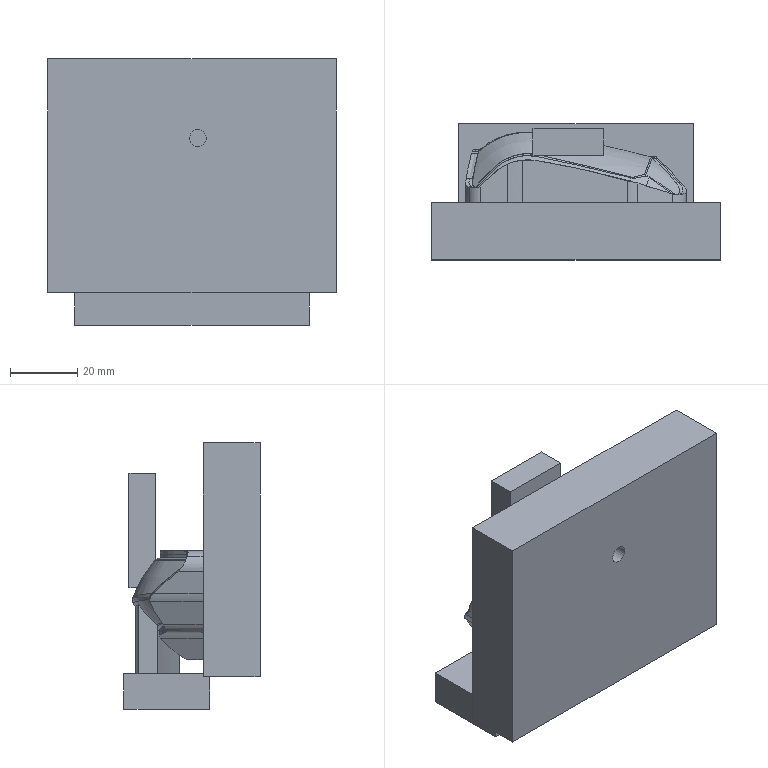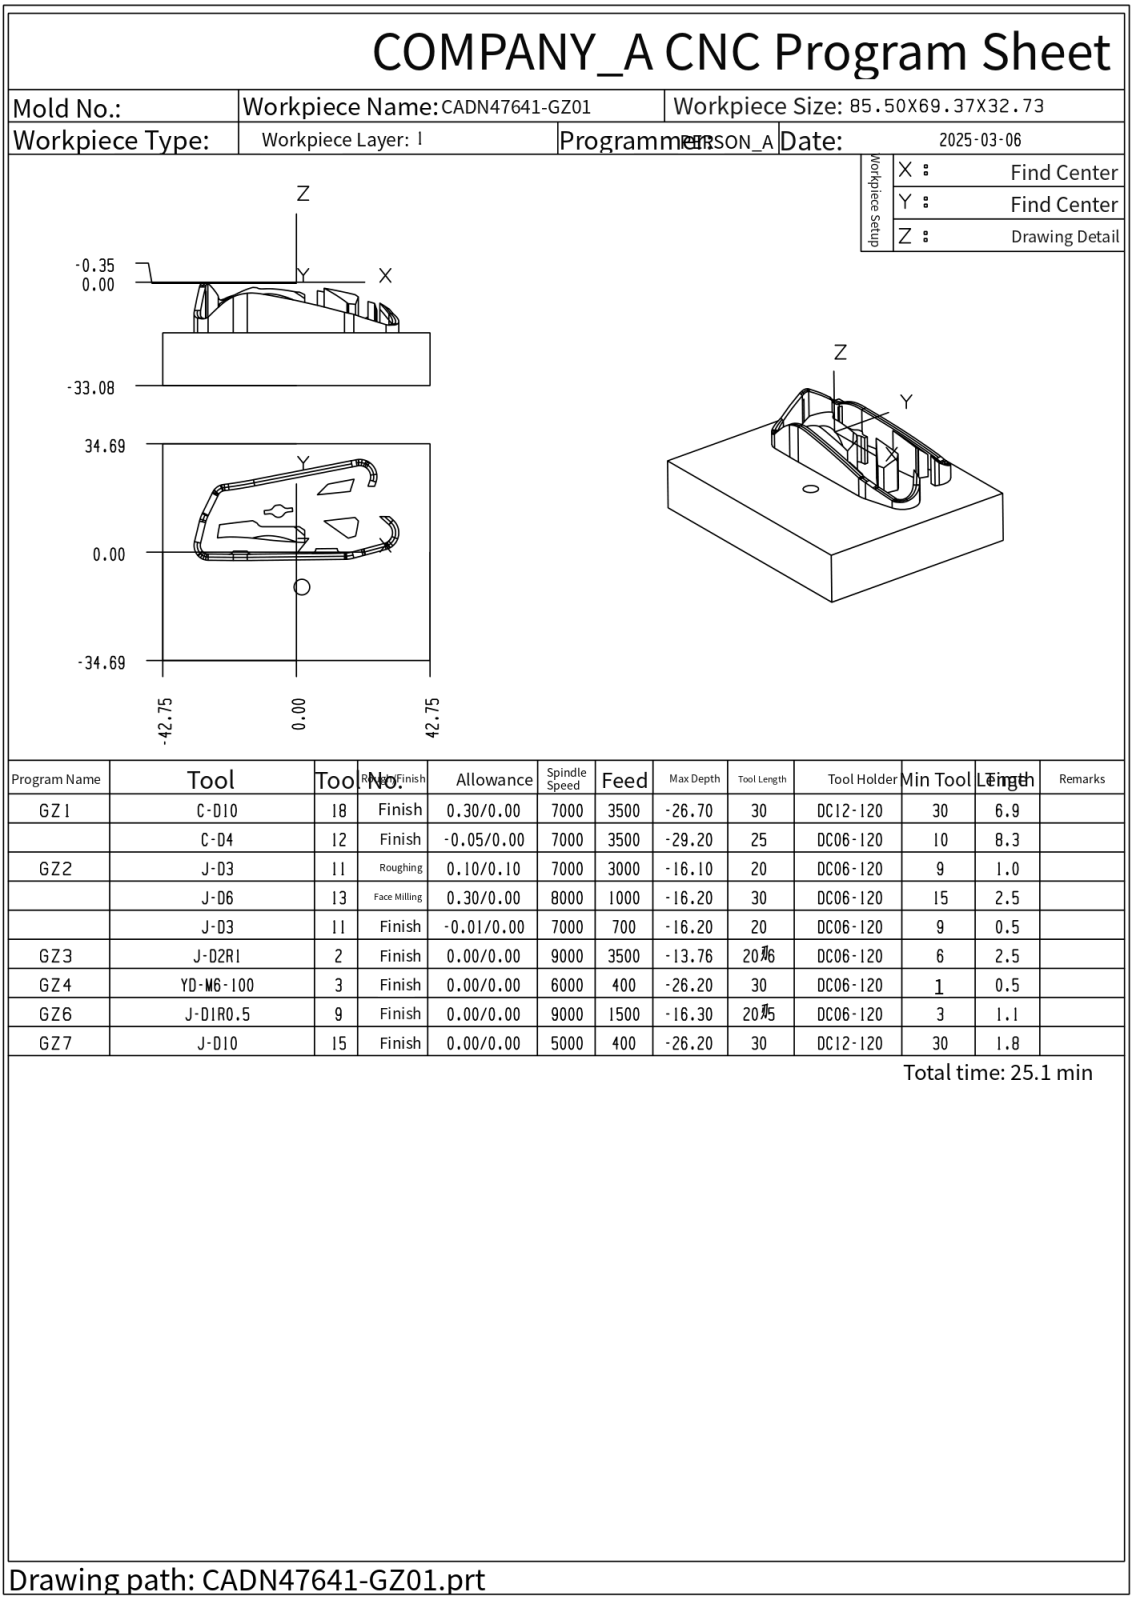NC program | NX | posted by the shop | part box 85.5 x 40.385 x 79 mm
Lines 36040 to 36898 of 71032:
36039 TOOL CALL 10 Z S7000
36040 CALL LBL101
36041 M3 M8
36042 M51
36043 CYCL DEF 32.0 TOLERANCE
36044 CYCL DEF 32.1 T0.012
36045 CYCL DEF 32.2 HSC-MODE:0
36046 L M126
36047 PLANE SPATIAL SPA-90. SPB+0.0 SPC+180. TURN FMAX SEQ-
36048 L X24.8955 Y1.6366 FMAX
36049 L Z102.5 FMAX
36050 L Z8.2072 FMAX
36051 L Z7.2072 F1500.
36052 CC X25.3717 Y2.5159
36053 C X26.2511 Y2.0397 DR+
36054 CC X27.7805 Y1.2115
36055 C X26.3392 Y2.1851 DR- F3000.
36056 L X26.3096 Y2.2798
36057 L X26.2417 Y2.5151
36058 L X26.1261 Y2.3992 Z7.1574
36059 L X26.0636 Y2.3031 Z7.1076
36060 L X26.1734 Y2.0672
36061 CC X27.7778 Y1.1917
36062 C X26.084 Y1.8786 DR+
36063 L X26.0215 Y1.8443 Z7.0579
36064 L X25.9513 Y1.813 Z7.0081
36065 CC X27.3487 Y1.2565
36066 C X26.0344 Y1.9878 DR-
36067 L X25.8966 Y2.2389
36068 L X25.8145 Y2.2304 Z6.9583
36069 L X25.7429 Y2.2281 Z6.9085
36070 L X25.797 Y2.1394
36071 L X25.9108 Y1.9375
36072 CC X27.42 Y1.2131
36073 C X25.8323 Y1.744 DR+
36074 L X25.7242 Y1.7093 Z6.8089
36075 CC X27.5017 Y1.1601
36076 C X25.7986 Y1.9087 DR-
36077 L X25.6495 Y2.143
36078 L X25.5344 Y2.1299 Z6.7094
36079 L X25.692 Y1.8917
36080 CC X27.1996 Y1.2027
36081 C X25.6196 Y1.7037 DR+
36082 L X25.5195 Y1.7021 Z6.6098
36083 CC X27.3098 Y1.2067
36084 C X25.5856 Y1.8979 DR-
36085 CC X33.768 Y7.9039
36086 C X25.4478 Y2.0903 DR-
36087 L X25.339 Y2.1081 Z6.5102
36088 L X25.489 Y1.8865
36089 CC X26.9832 Y1.2052
36090 C X25.4181 Y1.7025 DR+
36091 L X25.3164 Y1.6861 Z6.4106
36092 CC X27.0085 Y1.1978
36093 C X25.3883 Y1.888 DR-
36094 CC X39.6492 Y12.0493
36095 C X25.2447 Y2.0926 DR-
36096 L X25.1426 Y2.0958 Z6.3111
36097 CC X41.4267 Y13.3714
36098 C X25.2873 Y1.8897 DR+
36099 CC X26.8851 Y1.196
36100 C X25.2153 Y1.6919 DR+
36101 L X25.114 Y1.6927 Z6.2115
36102 CC X26.8865 Y1.1603
36103 C X25.1863 Y1.8914 DR-
36104 L X25.0346 Y2.1137
36105 L X24.938 Y2.1018 Z6.1119
36106 CC X43.0434 Y14.724
36107 C X25.0853 Y1.8931 DR+
36108 CC X26.6853 Y1.1961
36109 C X25.0125 Y1.6936 DR+
36110 L X24.9108 Y1.6893 Z6.0123
36111 CC X26.7839 Y1.1358
36112 C X24.9842 Y1.8947 DR-
36113 CC X43.0304 Y14.8684
36114 C X24.8355 Y2.1041 DR-
36115 L X24.7258 Y2.1236 Z5.9128
36116 L X24.8832 Y1.8963
36117 CC X26.4842 Y1.1965
36118 C X24.8094 Y1.6947 DR+
36119 L X24.7079 Y1.695 Z5.8132
36120 CC X26.385 Y1.1965
36121 C X24.7819 Y1.8974 DR-
36122 CC X46.4901 Y17.538
36123 C X24.6298 Y2.1107 DR-
36124 L X24.5174 Y2.1339 Z5.7136
36125 L X24.6805 Y1.8982
36126 CC X26.2829 Y1.1968
36127 C X24.6055 Y1.6929 DR+
36128 L X24.5528 Y1.698 Z5.6638
36129 L X24.5034 Y1.7028 Z5.614
36130 CC X26.0829 Y1.2061
36131 C X24.5791 Y1.8991 DR-
36132 L X24.4146 Y2.1348
36133 L X24.3127 Y2.1338 Z5.5145
36134 L X24.4766 Y1.9005
36135 CC X26.3028 Y1.1302
36136 C X24.4006 Y1.6872 DR+
36137 L X24.2982 Y1.6896 Z5.4149
36138 CC X26.2077 Y1.1283
36139 C X24.374 Y1.9021 DR-
36140 L X24.2106 Y2.1327
36141 L X24.1056 Y2.1354 Z5.3153
36142 L X24.2712 Y1.9035
36143 CC X25.8632 Y1.1994
36144 C X24.1945 Y1.6952 DR+
36145 L X24.0904 Y1.6843 Z5.2157
36146 CC X25.8194 Y1.2023
36147 C X24.1675 Y1.9045 DR-
36148 CC X52.3731 Y22.7661
36149 C X24.0075 Y2.1226 DR-
36150 L X23.8997 Y2.1319 Z5.1162
36151 L X24.0639 Y1.9054
36152 CC X25.8639 Y1.1348
36153 C X23.9869 Y1.6921 DR+
36154 L X23.9317 Y1.6946 Z5.0664
36155 L X23.8831 Y1.6967 Z5.0166
36156 CC X25.558 Y1.1996
36157 C X23.9603 Y1.9064 DR-
36158 L X23.7961 Y2.1315
36159 L X23.6907 Y2.1351 Z4.917
36160 L X23.8567 Y1.9074
36161 CC X25.4562 Y1.1996
36162 C X23.7791 Y1.6964 DR+
36163 L X23.675 Z4.8174
36164 CC X25.3517 Y1.1999
36165 C X23.7531 Y1.9084 DR-
36166 CC X-14.5661 Y-25.5947
36167 C X23.5828 Y2.1441 DR+
36168 L X23.4754 Y2.1519 Z4.7179
36169 CC X6.3711 Y-10.3123
36170 C X23.6495 Y1.9095 DR-
36171 CC X25.2481 Y1.2001
36172 C X23.571 Y1.6963 DR+
36173 L X23.4661 Y1.6939 Z4.6183
36174 CC X25.1407 Y1.2006
36175 C X23.5459 Y1.9105 DR-
36176 L X23.3701 Y2.1518
36177 L X23.2597 Y2.1585 Z4.5187
36178 L X23.4422 Y1.9115
36179 CC X25.0281 Y1.2006
36180 C X23.3603 Y1.6892 DR+
36181 L X23.2545 Y1.6872 Z4.4192
36182 CC X24.9323 Y1.2016
36183 C X23.3369 Y1.9127 DR-
36184 CC X-1.8278 Y-16.8967
36185 C X23.1545 Y2.1544 DR+
36186 L X23.0463 Y2.1564 Z4.3196
36187 CC X1.77 Y-14.2955
36188 C X23.2316 Y1.9139 DR-
36189 CC X25.0476 Y1.1316
36190 C X23.1486 Y1.6829 DR+
36191 L X23.0416 Y1.6845 Z4.22
36192 CC X24.7127 Y1.2029
36193 C X23.1258 Y1.9145 DR-
36194 CC X12.7774 Y-5.7107
36195 C X22.9256 Y2.179 DR+
36196 L X22.818 Y2.1742 Z4.1204
36197 CC X10.7984 Y-7.3342
36198 C X23.0192 Y1.9142 DR-
36199 CC X24.4819 Y1.2153
36200 C X22.9339 Y1.6967 DR+
36201 L X22.8259 Y1.6771 Z4.0209
36202 CC X24.4887 Y1.2027
36203 C X22.9125 Y1.9139 DR-
36204 CC X14.3973 Y-4.4789
36205 C X22.702 Y2.1851 DR+
36206 L X22.6044 Y2.1613 Z3.9213
36207 CC X10.6334 Y-7.7466
36208 C X22.8045 Y1.9144 DR-
36209 CC X24.238 Y1.2167
36210 C X22.7182 Y1.6983 DR+
36211 L X22.6063 Y1.6673 Z3.8217
36212 CC X24.2788 Y1.205
36213 C X22.6958 Y1.9155 DR-
36214 CC X15.3362 Y-3.7929
36215 C X22.4727 Y2.1921 DR+
36216 L X22.3547 Y2.1969 Z3.7221
36217 CC X15.6882 Y-3.55
36218 C X22.5868 Y1.9161 DR-
36219 CC X24.1608 Y1.2043
36220 C X22.4946 Y1.6606 DR+
36221 L X22.383 Y1.6581 Z3.6226
36222 CC X24.0143 Y1.211
36223 C X22.4759 Y1.914 DR-
36224 CC X16.2269 Y-3.0782
36225 C X22.2405 Y2.1952 DR+
36226 L X22.1209 Y2.196 Z3.523
36227 CC X16.4218 Y-2.9462
36228 C X22.365 Y1.9119 DR-
36229 CC X24.4735 Y1.0454
36230 C X22.2684 Y1.6235 DR+
36231 L X22.2135 Y1.6281 Z3.4732
36232 L X22.1524 Y1.6331 Z3.4234
36233 CC X23.7678 Y1.2112
36234 C X22.2516 Y1.9104 DR-
36235 CC X16.4952 Y-2.9147
36236 C X21.9929 Y2.2032 DR+
36237 L X21.8711 Y2.2002 Z3.3238
36238 CC X16.515 Y-2.9538
36239 C X22.1363 Y1.9095 DR-
36240 CC X23.6864 Y1.2123
36241 C X22.0357 Y1.617 DR+
36242 L X21.9832 Y1.621 Z3.2741
36243 L X21.9192 Y1.6259 Z3.2243
36244 CC X23.5139 Y1.2118
36245 C X22.0208 Y1.9083 DR-
36246 CC X16.5828 Y-2.9487
36247 C X21.7491 Y2.1964 DR+
36248 L X21.6213 Y2.1893 Z3.1247
36249 CC X15.2422 Y-4.4418
36250 C X21.9036 Y1.9056 DR-
36251 CC X23.3745 Y1.2115
36252 C X21.7979 Y1.6111 DR+
36253 L X21.676 Y1.5633 Z3.0251
36254 CC X23.3595 Y1.2036
36255 C X21.7864 Y1.9028 DR-
36256 CC X16.3602 Y-3.34
36257 C X21.4761 Y2.206 DR+
36258 L X21.364 Y2.1765 Z2.9255
36259 CC X15.043 Y-4.9679
36260 C X21.6638 Y1.8996 DR-
36261 CC X23.199 Y1.2006
36262 C X21.5553 Y1.5796 DR+
36263 L X21.4271 Y1.5614 Z2.826
36264 CC X23.0389 Y1.2097
36265 C X21.539 Y1.8966 DR-
36266 CC X16.0115 Y-3.928
36267 C X21.2034 Y2.1976 DR+
36268 L X21.1256 Y2.2076 Z2.7762
36269 L X21.044 Y2.213 Z2.7264
36270 CC X17.09 Y-2.7001
36271 C X21.4127 Y1.892 DR-
36272 CC X22.8976 Y1.2075
36273 C X21.2973 Y1.5432 DR+
36274 L X21.2325 Y1.5413 Z2.6766
36275 L X21.1674 Y1.5394 Z2.6268
36276 CC X22.7246 Y1.2057
36277 C X21.2845 Y1.8859 DR-
36278 CC X16.3127 Y-3.7358
36279 C X20.9148 Y2.1923 DR+
36280 L X20.8438 Y2.192 Z2.577
36281 L X20.7692 Y2.187 Z2.5272
36282 CC X16.8294 Y-3.1385
36283 C X21.1542 Y1.8794 DR-
36284 CC X22.5922 Y1.205
36285 C X21.0365 Y1.5251 DR+
36286 L X20.9669 Y1.5 Z2.4775
36287 L X20.8978 Y1.4747 Z2.4277
36288 CC X22.5262 Y1.2043
36289 C X21.0171 Y1.8732 DR-
36290 CC X16.7702 Y-3.2507
36291 C X20.6072 Y2.187 DR+
36292 L X20.5297 Y2.1862 Z2.3779
36293 L X20.449 Y2.1808 Z2.3281
36294 CC X16.723 Y-3.3841
36295 C X20.8796 Y1.867 DR-
36296 CC X22.2455 Y1.2033
36297 C X20.7555 Y1.4967 DR+
36298 L X20.6775 Y1.4875 Z2.2783
36299 L X20.6106 Y1.4761 Z2.2285
36300 CC X22.0897 Y1.1998
36301 C X20.7376 Y1.8599 DR-
36302 CC X16.3511 Y-4.0036
36303 C X20.2744 Y2.1795 DR+
36304 L X20.1978 Y2.1727 Z2.1787
36305 L X20.1182 Y2.1612 Z2.129
36306 CC X15.7622 Y-5.0156
36307 C X20.5933 Y1.8503 DR-
36308 CC X21.9683 Y1.1963
36309 C X20.4662 Y1.4456 DR+
36310 L X20.3884 Y1.4336 Z2.0792
36311 L X20.3209 Y1.4199 Z2.0294
36312 CC X21.8815 Y1.1977
36313 C X20.4425 Y1.8411 DR-
36314 CC X16.212 Y-4.3432
36315 C X19.9557 Y2.1473 DR+
36316 L X19.8655 Y2.1439 Z1.9796
36317 L X19.7731 Y2.1364 Z1.9298
36318 CC X15.6636 Y-5.3909
36319 C X20.2883 Y1.8313 DR-
36320 CC X21.6455 Y1.1962
36321 C X20.1601 Y1.3939 DR+
36322 L X20.0692 Y1.3996 Z1.88
36323 L X19.9965 Y1.4041 Z1.8302
36324 CC X21.4189 Y1.1858
36325 C X20.1279 Y1.8214 DR-
36326 CC X16.4847 Y-3.9749
36327 C X19.5825 Y2.1303 DR+
36328 L X19.5031 Y2.1175 Z1.7804
36329 L X19.4219 Y2.1009 Z1.7307
36330 CC X16.11 Y-4.7151
36331 C X19.9624 Y1.8107 DR-
36332 CC X21.2876 Y1.1796
36333 C X19.8345 Y1.3871 DR+
36334 L X19.7466 Y1.3778 Z1.6809
36335 L X19.6662 Y1.3675 Z1.6311
36336 CC X21.1125 Y1.1767
36337 C X19.7934 Y1.7999 DR-
36338 CC X15.6865 Y-5.6573
36339 C X19.2476 Y2.0754 DR+
36340 L X19.1513 Y2.0682 Z1.5813
36341 L X19.0546 Y2.0601 Z1.5315
36342 CC X15.3276 Y-6.4919
36343 C X19.6171 Y1.7923 DR-
36344 CC X20.8571 Y1.187
36345 C X19.4896 Y1.3712 DR+
36346 L X19.3836 Y1.36 Z1.4815
36347 L X19.2953 Y1.3506 Z1.4315
36348 CC X20.7028 Y1.1833
36349 C X19.4179 Y1.7818 DR-
36350 CC X15.4281 Y-6.3559
36351 C X18.834 Y2.0429 DR+
36352 L X18.7398 Y2.0287 Z1.3815
36353 L X18.6442 Y2.0108 Z1.3315
36354 CC X14.683 Y-8.3264
36355 C X19.2262 Y1.7686 DR-
36356 CC X20.5094 Y1.1784
36357 C X19.1067 Y1.3437 DR+
36358 L X19.0013 Y1.3284 Z1.2815
36359 L X18.8998 Y1.3137 Z1.2315
36360 CC X20.2832 Y1.197
36361 C X19.014 Y1.7597 DR-
36362 CC X14.1995 Y-9.874
36363 C X18.4142 Y1.9902 DR+
36364 L X18.3087 Y1.9791 Z1.1815
36365 L X18.1998 Y1.9579 Z1.1315
36366 CC X13.469 Y-12.3197
36367 C X18.7953 Y1.7466 DR-
36368 CC X20.0777 Y1.1937
36369 C X18.6858 Y1.308 DR+
36370 L X18.5782 Y1.2926 Z1.0815
36371 L X18.4657 Y1.2765 Z1.0315
36372 CC X19.8461 Y1.1892
36373 C X18.5732 Y1.7304 DR-
36374 CC X12.9417 Y-14.567
36375 C X17.9606 Y1.9293 DR+
36376 L X17.868 Y1.9315 Z.9982
36377 L X17.7727 Y1.9243 Z.9648
36378 L X17.6775 Y1.917 Z.9315
36379 CC X14.6835 Y-9.0695
36380 C X18.3307 Y1.7178 DR-
36381 CC X19.6265 Y1.202
36382 C X18.2328 Y1.2543 DR+
36383 L X18.1102 Y1.2385 Z.8815
36384 L X17.9775 Y1.2214 Z.8315
36385 CC X19.3484 Y1.2017
36386 C X18.0722 Y1.7029 DR-
36387 CC X12.8002 Y-16.2613
36388 C X17.4204 Y1.8815 DR+
36389 L X17.3247 Y1.8752 Z.7982
36390 L X17.228 Y1.8648 Z.7648
36391 L X17.1312 Y1.8534 Z.7315
36392 CC X13.994 Y-12.2062
36393 C X17.8124 Y1.6838 DR-
36394 CC X19.0577 Y1.1906
36395 C X17.7183 Y1.1954 DR+
36396 L X17.5837 Y1.1765 Z.6815
36397 L X17.4321 Y1.1552 Z.6315
36398 CC X18.8845 Y1.1988
36399 C X17.5088 Y1.6666 DR-
36400 L X17.2415 Y1.7336
36401 L X16.8502 Y1.8072
36402 L X16.7445 Y1.8025 Z.5982
36403 L X16.6373 Y1.7902 Z.5648
36404 L X16.5299 Y1.7761 Z.5315
36405 CC X11.3526 Y-27.6509
36406 C X17.2129 Y1.6477 DR-
36407 CC X18.4403 Y1.1985
36408 C X17.1349 Y1.1335 DR+
36409 L X16.9452 Y1.1091 Z.4821
36410 L X16.7844 Y1.0886 Z.4328
36411 CC X18.0507 Y1.1999
36412 C X16.8524 Y1.6238 DR-
36413 L X16.678 Y1.6584
36414 L X16.162 Y1.7294
36415 L X16.0563 Y1.7271 Z.4081
36416 L X15.9497 Y1.7179 Z.3834
36417 L X15.8429 Y1.7069 Z.3587
36418 L X15.736 Y1.6949 Z.334
36419 CC X11.6675 Y-32.4141
36420 C X16.4749 Y1.5986 DR-
36421 CC X17.6471 Y1.1903
36422 C X16.4113 Y1.0745 DR+
36423 L X16.1834 Y1.0708 Z.2847
36424 L X15.9657 Y1.0672 Z.2353
36425 CC X17.0647 Y1.1989
36426 C X16.0222 Y1.5708 DR-
36427 CC X10.9722 Y-47.6625
36428 C X15.2909 Y1.6404 DR+
36429 L X15.1694 Y1.6278 Z.2106
36430 L X15.0477 Y1.6117 Z.1859
36431 L X14.9259 Y1.5957 Z.1612
36432 L X14.8037 Y1.5714 Z.1365
36433 L X15.2694 Y1.5538
36434 L X15.5005 Y1.5348
36435 CC X16.6876 Y1.2266
36436 C X15.4836 Y.9926 DR+
36437 CC X14.502 Y.8019
36438 C X14.6927 Y-.1798 DR-
36439 L Z1.1365
36440 L Z11.6923 FMAX
36441 L X28.5933 Y5.6856 F10000.
36442 L Z8.2072 FMAX
36443 L Z7.2072 F1500.
36444 CC X29.2913 Y4.9696
36445 C X28.5753 Y4.2715 DR+
36446 CC X27.2359 Y2.9659
36447 C X28.7776 Y4.0249 DR- F3000.
36448 CC X29.0636 Y6.0509
36449 C X29.3278 Y4.022 DR+
36450 L X29.3899 Y4.0662 Z7.1574
36451 L X29.4516 Y4.113 Z7.1076
36452 L X29.3559 Y4.1072
36453 CC X29.2696 Y5.1375
36454 C X29.0018 Y4.1388 DR-
36455 CC X27.9022 Y3.6327
36456 C X28.8866 Y4.3371 DR+
36457 L X28.9658 Y4.3912 Z7.0579
36458 L X29.0391 Y4.4413 Z7.0081
36459 CC X28.0269 Y3.7013
36460 C X29.1639 Y4.23 DR-
36461 CC X29.432 Y5.0372
36462 C X29.498 Y4.1892 DR+
36463 CC X29.6697 Y1.9821
36464 C X29.6155 Y4.1952 DR-
36465 L X29.6185 Y4.2308 Z6.9583
36466 L X29.6216 Y4.2667 Z6.9085
36467 CC X29.6187 Y1.6606
36468 C X29.4498 Y4.2613 DR+
36469 L X29.2844 Y4.3076
36470 L X29.2462 Y4.3858
36471 L X29.1363 Y4.5334
36472 L X29.2173 Y4.5518 Z6.8587
36473 L X29.2817 Y4.5586 Z6.8089
36474 CC X28.1765 Y3.8131
36475 C X29.382 Y4.3825 DR-
36476 L X29.4443 Y4.36
36477 CC X29.8709 Y6.4386
36478 C X29.7986 Y4.3179 DR+
36479 L X29.77 Y4.3977 Z6.7094
36480 L X29.6376 Y4.4008
36481 CC X29.6242 Y4.7303
36482 C X29.4587 Y4.4451 DR-
36483 CC X28.4493 Y3.9997
36484 C X29.3681 Y4.6104 DR+
36485 L X29.398 Y4.6405 Z6.6596
36486 L X29.4291 Y4.6717 Z6.6098
36487 CC X28.6175 Y4.0992
36488 C X29.5238 Y4.5054 DR-
36489 CC X29.6446 Y4.6706
36490 C X29.6376 Y4.4661 DR+
36491 L X29.7785 Y4.461
36492 CC X20.6695 Y-82.9604
36493 C X29.9096 Y4.4473 DR-
36494 L X29.8666 Y4.5179 Z6.5102
36495 CC X29.3458 Y-1.6371
36496 C X29.6376 Y4.533 DR+
36497 L X29.5913 Y4.5594
36498 L X29.5865 Y4.5593
36499 CC X28.4884 Y3.9865
36500 C X29.4906 Y4.7142 DR+
36501 L X29.5218 Y4.7731 Z6.4106
36502 CC X27.6309 Y3.2691
36503 C X29.634 Y4.62 DR-
36504 CC X29.7112 Y4.7067
36505 C X29.7141 Y4.5906 DR+
36506 L X29.7785 Y4.588
36507 L X29.9377 Y4.5757
36508 L X30.0164 Y4.5986 Z6.3608
36509 L X30.094 Y4.6375 Z6.3111
36510 CC X30.5563 Y2.2835
36511 C X30.0607 Y4.6307 DR+
36512 L X29.7785 Y4.6515
36513 L X29.71 Y4.6541
36514 L X29.5441 Y4.8375
36515 L X29.5278 Y4.9264 Z6.2115
36516 L X29.7137 Y4.7211
36517 L X30.0146 Y4.6991
36518 CC X30.5758 Y2.8323
36519 C X30.1067 Y4.7244 DR-
36520 L X30.1436 Y4.813 Z6.1119
36521 CC X30.7465 Y2.1282
36522 C X29.9757 Y4.7697 DR+
36523 L X29.7073 Y4.7892
36524 L X29.6376 Y4.8633
36525 L X29.5077 Y5.0104
36526 L X29.4743 Y5.1047 Z6.0123
36527 L X29.6376 Y4.9195
36528 L X29.6948 Y4.8575
36529 L X29.9311 Y4.8384
36530 CC X30.801 Y2.2297
36531 C X30.165 Y4.9051 DR-
36532 L X30.1448 Y4.9438 Z5.9625
36533 L X30.1263 Y4.9796 Z5.9128
36534 CC X30.9334 Y2.1156
36535 C X29.9066 Y4.9084 DR+
36536 L X29.6817 Y4.9259
36537 L X29.4597 Y5.178
36538 L X29.4282 Y5.2663 Z5.8132
36539 L X29.6651 Y4.9982
36540 L X29.8865 Y4.9804
36541 CC X31.1166 Y1.8536
36542 C X30.1271 Y5.0647 DR-
36543 L X30.13 Y5.1507 Z5.7136
36544 L X29.9194 Y5.0785
36545 L X29.8633 Y5.0562
36546 L X29.6469 Y5.0722
36547 L X29.5077 Y5.2282
36548 L X29.3981 Y5.3536
36549 L X29.3789 Y5.4325 Z5.614
36550 L X29.629 Y5.1461
36551 L X29.8439 Y5.1314
36552 L X30.1544 Y5.2406
36553 L X30.1466 Y5.3279 Z5.5145
36554 L X29.8177 Y5.2075
36555 L X29.7785 Y5.2121
36556 L X29.6107 Y5.2209
36557 L X29.3518 Y5.5179
36558 L X29.3259 Y5.6026 Z5.4149
36559 L X29.593 Y5.2958
36560 L X29.7911 Y5.2835
36561 L X30.1356 Y5.4134
36562 L X30.1071 Y5.456 Z5.3651
36563 L X30.0837 Y5.491 Z5.3153
36564 L X29.7645 Y5.3594
36565 L X29.5753 Y5.3707
36566 L X29.3002 Y5.6873
36567 L X29.2837 Y5.764 Z5.2157
36568 L X29.5577 Y5.4456
36569 L X29.7378 Y5.4353
36570 L X30.0802 Y5.5745
36571 L X30.0723 Y5.6196 Z5.166
36572 L X30.066 Y5.6557 Z5.1162
36573 L X29.7113 Y5.5111
36574 L X29.5399 Y5.5206
36575 CC X-14.3195 Y-31.6691
36576 C X29.2648 Y5.8427 DR+
36577 L X29.2358 Y5.9288 Z5.0166
36578 L X29.5219 Y5.5961
36579 L X29.6849 Y5.5874
36580 L X30.049 Y5.7356
36581 L X30.0202 Y5.7739 Z4.9668
36582 L X29.9951 Y5.8073 Z4.917
36583 L X29.6611 Y5.6634
36584 L X29.5038 Y5.6715
36585 L X29.4012 Y5.7898
36586 L X29.2147 Y6.0088
36587 L X29.1901 Y6.0926 Z4.8174
36588 L X29.4858 Y5.7474
36589 L X29.6404 Y5.74
36590 L X29.9856 Y5.8879
36591 L X29.9277 Y5.9588 Z4.7179
36592 CC X30.8405 Y3.5668
36593 C X29.6206 Y5.8178 DR+
36594 L X29.4671 Y5.8247
36595 L X29.1744 Y6.1678
36596 L X29.1548 Y6.2471 Z4.6183
36597 L X29.4484 Y5.902
36598 L X29.601 Y5.8955
36599 L X29.9452 Y6.0418
36600 L X29.9481 Y6.1231 Z4.5187
36601 L X29.5814 Y5.9732
36602 L X29.4297 Y5.9794
36603 L X29.1399 Y6.3228
36604 L X29.122 Y6.4009 Z4.4192
36605 L X29.4111 Y6.0567
36606 L X29.5619 Y6.0509
36607 L X29.9279 Y6.1997
36608 L X29.9036 Y6.2354 Z4.3694
36609 L X29.8789 Y6.2717 Z4.3196
36610 CC X30.9073 Y3.3952
36611 C X29.5433 Y6.1286 DR+
36612 L X29.3928 Y6.1342
36613 L X29.1055 Y6.478
36614 L X29.0863 Y6.5571 Z4.22
36615 L X29.3559 Y6.2337
36616 L X29.3745 Y6.2119
36617 L X29.525 Y6.2062
36618 L X29.9022 Y6.3554
36619 L X29.8905 Y6.3984 Z4.1702
36620 L X29.8814 Y6.4319 Z4.1204
36621 L X29.5067 Y6.2838
36622 L X29.3559 Y6.2903
36623 L X29.0693 Y6.6345
36624 L X29.0541 Y6.7106 Z4.0209
36625 L X29.3384 Y6.3679
36626 L X29.4883 Y6.3617
36627 L X29.8421 Y6.5054
36628 L X29.834 Y6.5448 Z3.9711
36629 L X29.8259 Y6.584 Z3.9213
36630 L X29.4706 Y6.4414
36631 L X29.3192 Y6.4474
36632 L X29.1637 Y6.6321
36633 L X29.0309 Y6.7939
36634 L X29.0214 Y6.8666 Z3.8217
36635 L X29.3 Y6.5269
36636 L X29.4529 Y6.5211
36637 L X29.8099 Y6.6627
36638 L X29.7607 Y6.7361 Z3.7221
36639 CC X30.5843 Y4.294
36640 C X29.4352 Y6.6008 DR+
36641 L X29.2809 Y6.6063
36642 L X28.9968 Y6.9516
36643 L X28.9772 Y7.0325 Z3.6226
36644 L X29.2617 Y6.6865
36645 L X29.4168 Y6.6809
36646 L X29.7771 Y6.8184
36647 L X29.7028 Y6.8886 Z3.523
36648 CC X30.3978 Y4.7964
36649 C X29.398 Y6.7612 DR+
36650 L X29.2424 Y6.7669
36651 L X28.9627 Y7.1093
36652 L X28.9408 Y7.1917 Z3.4234
36653 L X29.0742 Y7.0272
36654 L X29.2232 Y6.8473
36655 L X29.3809 Y6.8414
36656 L X29.723 Y6.9685
36657 L X29.7069 Y7.0049 Z3.3736
36658 L X29.6903 Y7.0423 Z3.3238
36659 CC X31.1196 Y2.6917
36660 C X29.3648 Y6.9215 DR+
36661 L X29.204 Y6.9278
36662 L X29.0742 Y7.0849
36663 L X28.9252 Y7.2689
36664 L X28.9092 Y7.3485 Z3.2243
36665 L X29.1848 Y7.0088
36666 L X29.3516 Y7.0012
36667 CC X30.6311 Y4.2129
36668 C X29.6599 Y7.123 DR-
36669 L X29.731 Y7.2187 Z3.1247
36670 L X29.3319 Y7.0818
36671 L X29.1656 Y7.0897
36672 L X28.8935 Y7.4279
36673 L X28.8753 Y7.5094 Z3.0251
36674 L X29.1464 Y7.1706
36675 L X29.3139 Y7.1627
36676 L X29.3999 Y7.1937
36677 L X29.7242 Y7.3036
36678 L X29.6474 Y7.3757 Z2.9255
36679 CC X31.0982 Y2.9594
36680 C X29.2983 Y7.2452 DR+
36681 L X29.1265 Y7.253
36682 L X28.8556 Y7.5926
36683 L X28.8361 Y7.6755 Z2.826
36684 L X29.1064 Y7.336
36685 L X29.2813 Y7.328
36686 CC X30.8376 Y3.7389
36687 C X29.6214 Y7.457 DR-
36688 L X29.6122 Y7.4969 Z2.7762
36689 L X29.6025 Y7.5394 Z2.7264
36690 L X29.2643 Y7.4107
36691 L X29.0863 Y7.419
36692 L X28.8167 Y7.7584
36693 L X28.7964 Y7.842 Z2.6268
36694 L X29.0663 Y7.5019
36695 L X29.2469 Y7.4935
36696 L X29.5834 Y7.6218
36697 L X29.5745 Y7.6607 Z2.577
36698 L X29.5645 Y7.7043 Z2.5272
36699 L X29.2289 Y7.5764
36700 L X29.0465 Y7.5851
36701 L X28.7772 Y7.925
36702 L X28.753 Y8.0131 Z2.4277
36703 L X28.9564 Y7.7553
36704 L X29.0266 Y7.6682
36705 L X29.2108 Y7.6593
36706 CC X28.281 Y10.7578
36707 C X29.5698 Y7.7906 DR+
36708 L X29.5505 Y7.8322 Z2.3779
36709 L X29.5326 Y7.8705 Z2.3281
36710 L X29.1927 Y7.7422
36711 L X29.0068 Y7.7513
36712 L X28.7352 Y8.0959
36713 L X28.7105 Y8.1845 Z2.2285
36714 L X28.7924 Y8.0788
36715 L X28.9865 Y7.8357
36716 L X29.1761 Y7.8261
36717 L X29.5163 Y7.9536
36718 L X29.4971 Y7.9907 Z2.1787
36719 L X29.4751 Y8.0334 Z2.129
36720 CC X29.9381 Y6.9529
36721 C X29.3559 Y7.9741 DR+
36722 L X29.1599 Y7.9102
36723 L X28.9662 Y7.9201
36724 L X28.7021 Y8.2595
36725 L X28.6817 Y8.3448 Z2.0294
36726 L X28.9206 Y8.0361
36727 L X28.9458 Y8.0045
36728 L X29.1436 Y7.9942
36729 L X29.3559 Y8.0632
36730 L X29.482 Y8.1202
36731 L X29.4745 Y8.1632 Z1.9796
36732 L X29.4673 Y8.2048 Z1.9298
36733 CC X29.9115 Y7.1775
36734 C X29.4399 Y8.1925 DR+
36735 L X29.3559 Y8.1535
36736 L X29.1272 Y8.0789
36737 L X28.9251 Y8.0898
36738 L X28.7924 Y8.2575
36739 L X28.6563 Y8.4344
36740 L X28.643 Y8.514 Z1.8302
36741 L X28.9042 Y8.1755
36742 L X29.0742 Y8.1681
36743 L X29.1108 Y8.1641
36744 L X29.215 Y8.1976
36745 L X29.4796 Y8.294
36746 L X29.4685 Y8.3443 Z1.7804
36747 L X29.461 Y8.378 Z1.7307
36748 L X29.0943 Y8.2493
36749 L X29.0742 Y8.2515
36750 L X28.8833 Y8.2612
36751 CC X88.7079 Y55.2401
36752 C X28.6127 Y8.6079 DR-
36753 L X28.5943 Y8.6935 Z1.6311
36754 L X28.667 Y8.5977
36755 L X28.8627 Y8.347
36756 L X29.0771 Y8.3347
36757 L X29.484 Y8.4754
36758 L X29.4125 Y8.5407 Z1.5315
36759 L X29.0579 Y8.4163
36760 L X28.8436 Y8.4284
36761 L X28.7924 Y8.4939
36762 L X28.5857 Y8.7651
36763 L X28.566 Y8.8558 Z1.4315
36764 L X28.8223 Y8.5189
36765 L X29.036 Y8.507
36766 CC X32.7314 Y-1.7133
36767 C X29.4066 Y8.6335 DR-
36768 L X29.3437 Y8.7125 Z1.3315
36769 CC X30.5692 Y4.8176
36770 C X29.0152 Y8.5935 DR+
36771 L X28.802 Y8.6052
36772 L X28.5896 Y8.8785
36773 L X28.5309 Y8.9561
36774 L X28.5237 Y9.0325 Z1.2315
36775 L X28.7804 Y8.6935
36776 L X28.9992 Y8.6814
36777 L X29.3172 Y8.7975
36778 L X29.3063 Y8.8384 Z1.1815
36779 L X29.2944 Y8.8833 Z1.1315
36780 L X28.9835 Y8.7693
36781 L X28.7924 Y8.7826
36782 L X28.7585 Y8.7822
36783 L X28.6837 Y8.8785
36784 L X28.4963 Y9.1263
36785 L X28.4805 Y9.2103 Z1.0315
36786 CC X-840.2096 Y-646.5419
36787 C X28.7366 Y8.871 DR-
36788 L X28.9678 Y8.8573
36789 L X29.2766 Y8.9707
36790 L X29.2671 Y9.0132 Z.9815
36791 L X29.257 Y9.0579 Z.9315
36792 L X28.9484 Y8.9459
36793 L X28.715 Y8.9597
36794 L X28.5622 Y9.1593
36795 L X28.4552 Y9.3026
36796 L X28.4406 Y9.3855 Z.8315
36797 L X28.6935 Y9.0485
36798 L X28.928 Y9.0346
36799 CC X27.9015 Y12.5835
36800 C X29.2611 Y9.1483 DR+
36801 L X29.1931 Y9.2294 Z.7315
36802 CC X29.6449 Y8.1485
36803 C X29.0742 Y9.1716 DR+
36804 L X28.9077 Y9.1233
36805 L X28.672 Y9.1373
36806 L X28.4218 Y9.4721
36807 L X28.4019 Y9.5602 Z.6315
36808 L X28.6506 Y9.2266
36809 L X28.8898 Y9.2126
36810 CC X27.2363 Y14.7677
36811 C X29.2271 Y9.3244 DR+
36812 L X29.2209 Y9.3769 Z.5815
36813 L X29.2171 Y9.41 Z.5315
36814 CC X27.0543 Y15.4461
36815 C X28.8744 Y9.2979 DR-
36816 L X28.6301 Y9.3116
36817 L X28.3797 Y9.6471
36818 L X28.3486 Y9.7481 Z.4328
36819 L X28.3687 Y9.7209
36820 L X28.6078 Y9.4045
36821 L X28.8575 Y9.3911
36822 L X29.1809 Y9.4994
36823 L X29.1786 Y9.5896 Z.334
36824 L X28.9333 Y9.5064
36825 L X28.8401 Y9.4803
36826 L X28.5858 Y9.4941
36827 L X28.4144 Y9.7209
36828 L X28.331 Y9.8336
36829 L X28.3177 Y9.9155 Z.2353
36830 L X28.5633 Y9.5843
36831 L X28.8213 Y9.5701
36832 L X29.1517 Y9.6761
36833 L X29.1484 Y9.732 Z.1859
36834 L X29.1462 Y9.768 Z.1365
36835 CC X62.3534 Y-96.4182
36836 C X28.8025 Y9.6598 DR+
36837 L X28.5407 Y9.6746
36838 L X28.2864 Y10.0146
36839 L X28.267 Y10.1033 Z.0378
36840 L X28.3418 Y10.0017
36841 L X28.5187 Y9.7649
36842 L X28.7837 Y9.7497
36843 L X29.1492 Y9.8617
36844 L X29.0907 Y9.9442 Z-.0609
36845 L X28.7625 Y9.8401
36846 L X28.497 Y9.8552
36847 L X28.2499 Y10.1899
36848 L X28.2284 Y10.2804 Z-.1597
36849 L X28.4753 Y9.9456
36850 L X28.7413 Y9.9304
36851 CC X30.4722 Y5.1107
36852 C X29.0509 Y10.0306 DR-
36853 L X29.0262 Y10.0744 Z-.2091
36854 L X29.0023 Y10.117 Z-.2584
36855 L X28.7197 Y10.0208
36856 L X28.4533 Y10.0364
36857 L X28.2066 Y10.3714
36858 L X28.1811 Y10.4659 Z-.3572
36859 L X28.316 Y10.2825
36860 L X28.4308 Y10.1282
36861 L X28.702 Y10.1124
36862 L X28.9802 Y10.2072
36863 L X28.9935 Y10.3018 Z-.4559
36864 CC X28.203 Y12.2757
36865 C X28.6849 Y10.2048 DR-
36866 L X28.4083 Y10.2199
36867 L X28.1631 Y10.5536
36868 L X28.1383 Y10.6473 Z-.5546
36869 L X28.229 Y10.5238
36870 L X28.3858 Y10.312
36871 L X28.6723 Y10.2983
36872 L X28.941 Y10.388
36873 L X28.9887 Y10.489 Z-.6534
36874 CC X28.5198 Y11.607
36875 C X28.3631 Y10.4048 DR-
36876 L X28.2457 Y10.5633
36877 L X28.118 Y10.7372
36878 L X28.0978 Y10.8275 Z-.7521
36879 L X28.3405 Y10.4977
36880 CC X28.4949 Y11.7146
36881 C X28.7924 Y10.5245 DR+
36882 L X28.9136 Y10.5728
36883 L X28.9016 Y10.6207 Z-.8015
36884 L X28.8906 Y10.6648 Z-.8509
36885 L X28.7924 Y10.622
36886 CC X28.4681 Y11.9171
36887 C X28.3177 Y10.5905 DR-
36888 L X28.229 Y10.7093
36889 L X28.0726 Y10.9224
36890 L X28.0519 Y11.0132 Z-.9496
36891 L X28.2948 Y10.6833
36892 L X28.5735 Y10.6719
36893 L X28.6516 Y10.6858
36894 L X28.8805 Y10.7585
36895 L X28.916 Y10.867 Z-1.0484
36896 L X28.6516 Y10.7846
36897 L X28.5651 Y10.7641